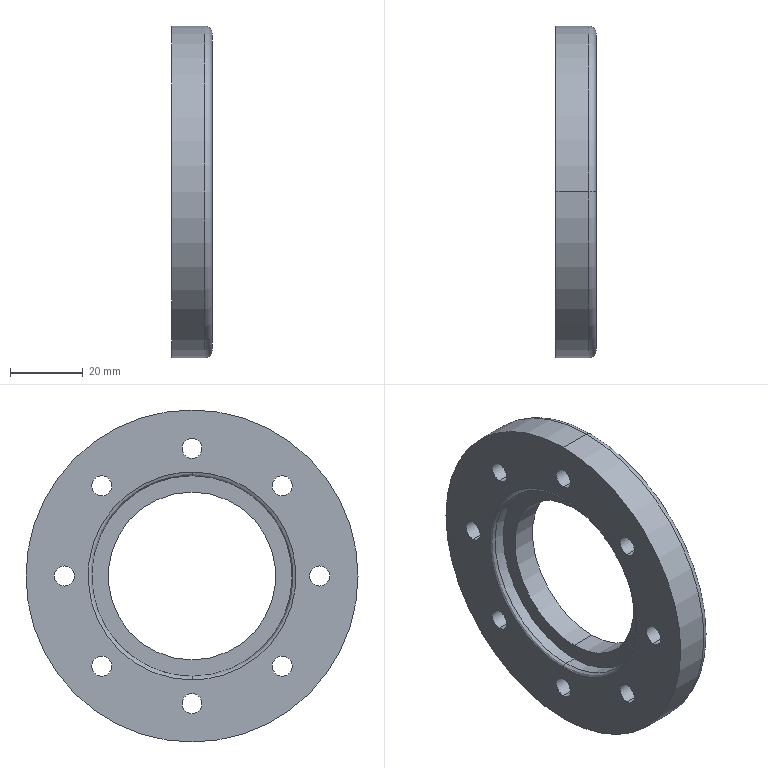Part | STEP file | 003.sldasm-Part-2_Valor predeterminado | 1 solid | 53 faces | box 11 x 91.038 x 91.038 mm | volume 45789 mm3 | cylinder 38 | plane 10 | spline 3 | torus 2 | commonest cylinder face diameters 5.5 x16 10 x16 46 x2 55 x2 91.038 x2